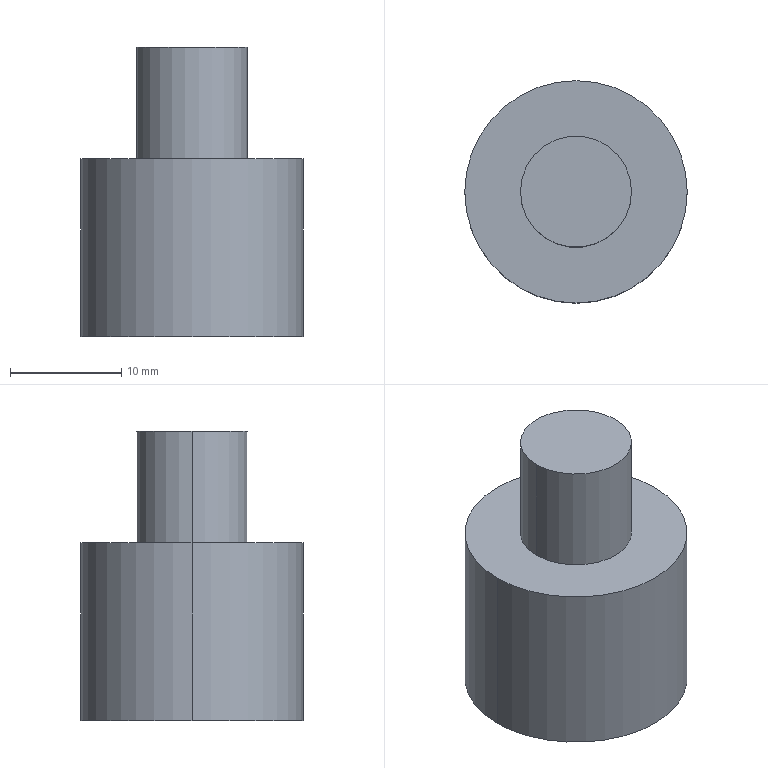Part | SolidWorks | features BaseBody 1 | 1 solid | 7 faces | box 20 x 20 x 26 mm | volume 5812 mm3 | cylinder 4 | plane 3 | commonest cylinder face diameters 10 x2 20 x2
STEP:
#1=CARTESIAN_POINT('',(-141.496,1845.044,-96.5));
#2=VERTEX_POINT('',#1);
#3=CARTESIAN_POINT('',(-161.496,1845.044,-96.5));
#4=VERTEX_POINT('',#3);
#5=CARTESIAN_POINT('',(-151.496,1845.044,-96.5));
#6=DIRECTION('',(0.,0.,1.));
#7=DIRECTION('',(1.,0.,0.));
#8=AXIS2_PLACEMENT_3D('',#5,#6,#7);
#9=CIRCLE('',#8,10.);
#10=EDGE_CURVE('',#2,#4,#9,.T.);
#11=ORIENTED_EDGE('',*,*,#10,.T.);
#12=CARTESIAN_POINT('',(-161.496,1845.044,-80.5));
#13=VERTEX_POINT('',#12);
#14=CARTESIAN_POINT('',(-161.496,1845.044,-96.5));
#15=DIRECTION('',(0.,0.,1.));
#16=VECTOR('',#15,1000.);
#17=LINE('',#14,#16);
#18=EDGE_CURVE('',#4,#13,#17,.T.);
#19=ORIENTED_EDGE('',*,*,#18,.T.);
#20=CARTESIAN_POINT('',(-141.496,1845.044,-80.5));
#21=VERTEX_POINT('',#20);
#22=CARTESIAN_POINT('',(-151.496,1845.044,-80.5));
#23=DIRECTION('',(0.,0.,-1.));
#24=DIRECTION('',(1.,0.,0.));
#25=AXIS2_PLACEMENT_3D('',#22,#23,#24);
#26=CIRCLE('',#25,10.);
#27=EDGE_CURVE('',#13,#21,#26,.T.);
#28=ORIENTED_EDGE('',*,*,#27,.T.);
#29=CARTESIAN_POINT('',(-141.496,1845.044,-96.5));
#30=DIRECTION('',(0.,0.,1.));
#31=VECTOR('',#30,1000.);
#32=LINE('',#29,#31);
#33=EDGE_CURVE('',#2,#21,#32,.T.);
#34=ORIENTED_EDGE('',*,*,#33,.F.);
#35=EDGE_LOOP('',(#11,#19,#28,#34));
#36=FACE_OUTER_BOUND('',#35,.T.);
#37=CARTESIAN_POINT('',(-151.496,1845.044,-96.5));
#38=DIRECTION('',(0.,0.,1.));
#39=DIRECTION('',(1.,0.,0.));
#40=AXIS2_PLACEMENT_3D('',#37,#38,#39);
#41=CYLINDRICAL_SURFACE('',#40,10.);
#42=ADVANCED_FACE('',(#36),#41,.T.);
#43=CARTESIAN_POINT('',(-146.496,1845.044,-80.5));
#44=VERTEX_POINT('',#43);
#45=CARTESIAN_POINT('',(-156.496,1845.044,-80.5));
#46=VERTEX_POINT('',#45);
#47=CARTESIAN_POINT('',(-151.496,1845.044,-80.5));
#48=DIRECTION('',(0.,0.,1.));
#49=DIRECTION('',(1.,0.,0.));
#50=AXIS2_PLACEMENT_3D('',#47,#48,#49);
#51=CIRCLE('',#50,5.);
#52=EDGE_CURVE('',#44,#46,#51,.T.);
#53=ORIENTED_EDGE('',*,*,#52,.T.);
#54=CARTESIAN_POINT('',(-156.496,1845.044,-70.5));
#55=VERTEX_POINT('',#54);
#56=CARTESIAN_POINT('',(-156.496,1845.044,-96.5));
#57=DIRECTION('',(0.,0.,1.));
#58=VECTOR('',#57,1000.);
#59=LINE('',#56,#58);
#60=EDGE_CURVE('',#46,#55,#59,.T.);
#61=ORIENTED_EDGE('',*,*,#60,.T.);
#62=CARTESIAN_POINT('',(-146.496,1845.044,-70.5));
#63=VERTEX_POINT('',#62);
#64=CARTESIAN_POINT('',(-151.496,1845.044,-70.5));
#65=DIRECTION('',(0.,0.,-1.));
#66=DIRECTION('',(1.,0.,0.));
#67=AXIS2_PLACEMENT_3D('',#64,#65,#66);
#68=CIRCLE('',#67,5.);
#69=EDGE_CURVE('',#55,#63,#68,.T.);
#70=ORIENTED_EDGE('',*,*,#69,.T.);
#71=CARTESIAN_POINT('',(-146.496,1845.044,-96.5));
#72=DIRECTION('',(0.,0.,1.));
#73=VECTOR('',#72,1000.);
#74=LINE('',#71,#73);
#75=EDGE_CURVE('',#44,#63,#74,.T.);
#76=ORIENTED_EDGE('',*,*,#75,.F.);
#77=EDGE_LOOP('',(#53,#61,#70,#76));
#78=FACE_OUTER_BOUND('',#77,.T.);
#79=CARTESIAN_POINT('',(-151.496,1845.044,-96.5));
#80=DIRECTION('',(0.,0.,1.));
#81=DIRECTION('',(1.,0.,0.));
#82=AXIS2_PLACEMENT_3D('',#79,#80,#81);
#83=CYLINDRICAL_SURFACE('',#82,5.);
#84=ADVANCED_FACE('',(#78),#83,.T.);
#85=ORIENTED_EDGE('',*,*,#18,.F.);
#86=CARTESIAN_POINT('',(-151.496,1845.044,-96.5));
#87=DIRECTION('',(0.,0.,1.));
#88=DIRECTION('',(1.,0.,0.));
#89=AXIS2_PLACEMENT_3D('',#86,#87,#88);
#90=CIRCLE('',#89,10.);
#91=EDGE_CURVE('',#4,#2,#90,.T.);
#92=ORIENTED_EDGE('',*,*,#91,.T.);
#93=ORIENTED_EDGE('',*,*,#33,.T.);
#94=CARTESIAN_POINT('',(-151.496,1845.044,-80.5));
#95=DIRECTION('',(0.,0.,-1.));
#96=DIRECTION('',(1.,0.,0.));
#97=AXIS2_PLACEMENT_3D('',#94,#95,#96);
#98=CIRCLE('',#97,10.);
#99=EDGE_CURVE('',#21,#13,#98,.T.);
#100=ORIENTED_EDGE('',*,*,#99,.T.);
#101=EDGE_LOOP('',(#85,#92,#93,#100));
#102=FACE_OUTER_BOUND('',#101,.T.);
#103=CARTESIAN_POINT('',(-151.496,1845.044,-96.5));
#104=DIRECTION('',(0.,0.,1.));
#105=DIRECTION('',(1.,0.,0.));
#106=AXIS2_PLACEMENT_3D('',#103,#104,#105);
#107=CYLINDRICAL_SURFACE('',#106,10.);
#108=ADVANCED_FACE('',(#102),#107,.T.);
#109=ORIENTED_EDGE('',*,*,#52,.F.);
#110=CARTESIAN_POINT('',(-151.496,1845.044,-80.5));
#111=DIRECTION('',(0.,0.,1.));
#112=DIRECTION('',(1.,0.,0.));
#113=AXIS2_PLACEMENT_3D('',#110,#111,#112);
#114=CIRCLE('',#113,5.);
#115=EDGE_CURVE('',#46,#44,#114,.T.);
#116=ORIENTED_EDGE('',*,*,#115,.F.);
#117=EDGE_LOOP('',(#109,#116));
#118=FACE_BOUND('',#117,.T.);
#119=ORIENTED_EDGE('',*,*,#99,.F.);
#120=ORIENTED_EDGE('',*,*,#27,.F.);
#121=EDGE_LOOP('',(#119,#120));
#122=FACE_OUTER_BOUND('',#121,.T.);
#123=CARTESIAN_POINT('',(-141.588,1843.687,-80.5));
#124=DIRECTION('',(0.,0.,-1.));
#125=DIRECTION('',(-1.,0.,0.));
#126=AXIS2_PLACEMENT_3D('',#123,#124,#125);
#127=PLANE('',#126);
#128=ADVANCED_FACE('',(#118,#122),#127,.F.);
#129=ORIENTED_EDGE('',*,*,#10,.F.);
#130=ORIENTED_EDGE('',*,*,#91,.F.);
#131=EDGE_LOOP('',(#129,#130));
#132=FACE_OUTER_BOUND('',#131,.T.);
#133=CARTESIAN_POINT('',(-151.496,1845.044,-96.5));
#134=DIRECTION('',(0.,0.,1.));
#135=DIRECTION('',(1.,0.,0.));
#136=AXIS2_PLACEMENT_3D('',#133,#134,#135);
#137=PLANE('',#136);
#138=ADVANCED_FACE('',(#132),#137,.F.);
#139=ORIENTED_EDGE('',*,*,#60,.F.);
#140=ORIENTED_EDGE('',*,*,#115,.T.);
#141=ORIENTED_EDGE('',*,*,#75,.T.);
#142=CARTESIAN_POINT('',(-151.496,1845.044,-70.5));
#143=DIRECTION('',(0.,0.,-1.));
#144=DIRECTION('',(1.,0.,0.));
#145=AXIS2_PLACEMENT_3D('',#142,#143,#144);
#146=CIRCLE('',#145,5.);
#147=EDGE_CURVE('',#63,#55,#146,.T.);
#148=ORIENTED_EDGE('',*,*,#147,.T.);
#149=EDGE_LOOP('',(#139,#140,#141,#148));
#150=FACE_OUTER_BOUND('',#149,.T.);
#151=CARTESIAN_POINT('',(-151.496,1845.044,-96.5));
#152=DIRECTION('',(0.,0.,1.));
#153=DIRECTION('',(1.,0.,0.));
#154=AXIS2_PLACEMENT_3D('',#151,#152,#153);
#155=CYLINDRICAL_SURFACE('',#154,5.);
#156=ADVANCED_FACE('',(#150),#155,.T.);
#157=ORIENTED_EDGE('',*,*,#147,.F.);
#158=ORIENTED_EDGE('',*,*,#69,.F.);
#159=EDGE_LOOP('',(#157,#158));
#160=FACE_OUTER_BOUND('',#159,.T.);
#161=CARTESIAN_POINT('',(-146.542,1844.366,-70.5));
#162=DIRECTION('',(0.,0.,-1.));
#163=DIRECTION('',(-1.,0.,0.));
#164=AXIS2_PLACEMENT_3D('',#161,#162,#163);
#165=PLANE('',#164);
#166=ADVANCED_FACE('',(#160),#165,.F.);
#167=CLOSED_SHELL('',(#42,#84,#108,#128,#138,#156,#166));
#168=MANIFOLD_SOLID_BREP('',#167);
#169=CARTESIAN_POINT('',(0.,0.,0.));
#170=DIRECTION('',(0.,0.,1.));
#171=DIRECTION('',(1.,0.,0.));
#172=AXIS2_PLACEMENT_3D('',#169,#170,#171);
#173=(LENGTH_UNIT()NAMED_UNIT(*)SI_UNIT(.MILLI.,.METRE.));
#174=UNCERTAINTY_MEASURE_WITH_UNIT(LENGTH_MEASURE(0.00001),#173,'','');
#175=(NAMED_UNIT(*)PLANE_ANGLE_UNIT()SI_UNIT($,.RADIAN.));
#176=(NAMED_UNIT(*)SI_UNIT($,.STERADIAN.)SOLID_ANGLE_UNIT());
#177=(GEOMETRIC_REPRESENTATION_CONTEXT(3)GLOBAL_UNCERTAINTY_ASSIGNED_CONTEXT((#174))GLOBAL_UNIT_ASSIGNED_CONTEXT((#173,#175,#176))REPRESENTATION_CONTEXT('',''));
#178=ADVANCED_BREP_SHAPE_REPRESENTATION('',(#168,#172),#177);